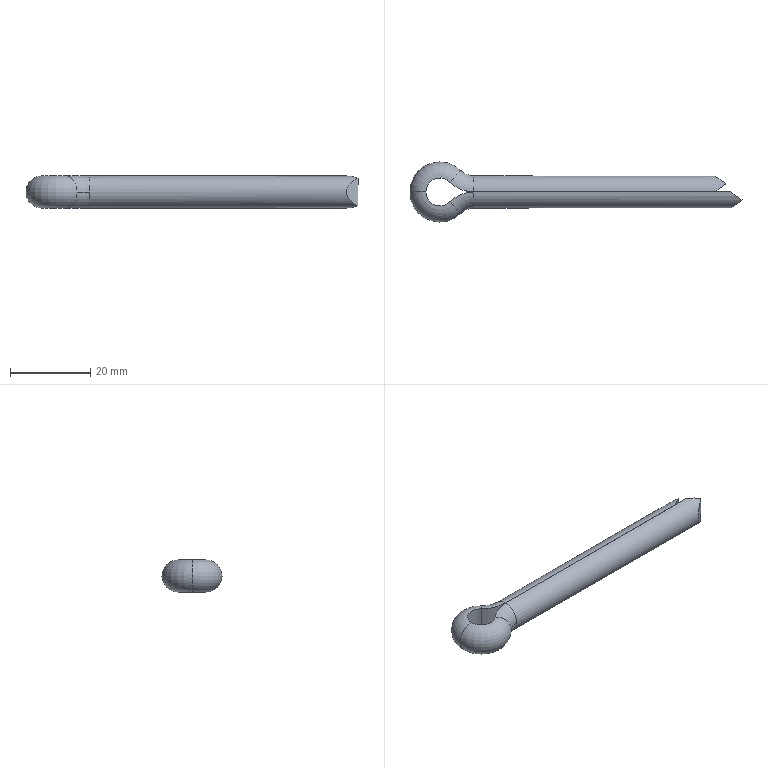Part | SolidWorks | features Cut 1, Sweep 1 | 1 solid | 17 faces | box 83 x 15 x 8 mm | volume 4081 mm3 | torus 6 | plane 6 | cylinder 5 | commonest cylinder face diameters 8 x2 17.139 x2 7.004 x1
STEP:
#1=CARTESIAN_POINT('',(0.,4.,0.));
#2=VERTEX_POINT('',#1);
#3=CARTESIAN_POINT('',(0.,0.002,4.));
#4=VERTEX_POINT('',#3);
#5=CARTESIAN_POINT('',(0.,0.,0.));
#6=DIRECTION('',(1.,0.,0.));
#7=DIRECTION('',(0.,0.,-1.));
#8=AXIS2_PLACEMENT_3D('',#5,#6,#7);
#9=CIRCLE('',#8,4.);
#10=EDGE_CURVE('',#2,#4,#9,.T.);
#11=ORIENTED_EDGE('',*,*,#10,.F.);
#12=CARTESIAN_POINT('',(-3.219,5.325,0.));
#13=VERTEX_POINT('',#12);
#14=CARTESIAN_POINT('',(0.,8.571,0.));
#15=DIRECTION('',(0.,0.,-1.));
#16=DIRECTION('',(-1.,0.,0.));
#17=AXIS2_PLACEMENT_3D('',#14,#15,#16);
#18=CIRCLE('',#17,4.571);
#19=EDGE_CURVE('',#2,#13,#18,.T.);
#20=ORIENTED_EDGE('',*,*,#19,.T.);
#21=CARTESIAN_POINT('',(-6.034,2.487,4.));
#22=VERTEX_POINT('',#21);
#23=CARTESIAN_POINT('',(-6.036,2.485,0.));
#24=DIRECTION('',(0.7101,-0.7041,0.));
#25=DIRECTION('',(0.,0.,-1.));
#26=AXIS2_PLACEMENT_3D('',#23,#24,#25);
#27=CIRCLE('',#26,4.);
#28=EDGE_CURVE('',#13,#22,#27,.T.);
#29=ORIENTED_EDGE('',*,*,#28,.T.);
#30=CARTESIAN_POINT('',(0.,8.571,4.));
#31=DIRECTION('',(0.,0.,-1.));
#32=DIRECTION('',(-1.,0.,0.));
#33=AXIS2_PLACEMENT_3D('',#30,#31,#32);
#34=CIRCLE('',#33,8.569);
#35=EDGE_CURVE('',#4,#22,#34,.T.);
#36=ORIENTED_EDGE('',*,*,#35,.F.);
#37=EDGE_LOOP('',(#11,#20,#29,#36));
#38=FACE_OUTER_BOUND('',#37,.T.);
#39=CARTESIAN_POINT('',(0.,8.571,0.));
#40=DIRECTION('',(0.,0.,-1.));
#41=DIRECTION('',(-1.,0.,0.));
#42=AXIS2_PLACEMENT_3D('',#39,#40,#41);
#43=TOROIDAL_SURFACE('',#42,8.571,4.);
#44=ADVANCED_FACE('',(#38),#43,.T.);
#45=CARTESIAN_POINT('',(-3.219,-5.325,0.));
#46=VERTEX_POINT('',#45);
#47=CARTESIAN_POINT('',(-6.034,-2.487,4.));
#48=VERTEX_POINT('',#47);
#49=CARTESIAN_POINT('',(-6.036,-2.485,0.));
#50=DIRECTION('',(-0.7101,-0.7041,0.));
#51=DIRECTION('',(0.,0.,-1.));
#52=AXIS2_PLACEMENT_3D('',#49,#50,#51);
#53=CIRCLE('',#52,4.);
#54=EDGE_CURVE('',#46,#48,#53,.T.);
#55=ORIENTED_EDGE('',*,*,#54,.F.);
#56=CARTESIAN_POINT('',(0.,-4.,0.));
#57=VERTEX_POINT('',#56);
#58=CARTESIAN_POINT('',(0.,-8.571,0.));
#59=DIRECTION('',(0.,0.,-1.));
#60=DIRECTION('',(-1.,0.,0.));
#61=AXIS2_PLACEMENT_3D('',#58,#59,#60);
#62=CIRCLE('',#61,4.571);
#63=EDGE_CURVE('',#46,#57,#62,.T.);
#64=ORIENTED_EDGE('',*,*,#63,.T.);
#65=CARTESIAN_POINT('',(0.,-0.002,4.));
#66=VERTEX_POINT('',#65);
#67=CARTESIAN_POINT('',(0.,0.,0.));
#68=DIRECTION('',(-1.,0.,0.));
#69=DIRECTION('',(0.,0.,-1.));
#70=AXIS2_PLACEMENT_3D('',#67,#68,#69);
#71=CIRCLE('',#70,4.);
#72=EDGE_CURVE('',#57,#66,#71,.T.);
#73=ORIENTED_EDGE('',*,*,#72,.T.);
#74=CARTESIAN_POINT('',(0.,-8.571,4.));
#75=DIRECTION('',(0.,0.,-1.));
#76=DIRECTION('',(-1.,0.,0.));
#77=AXIS2_PLACEMENT_3D('',#74,#75,#76);
#78=CIRCLE('',#77,8.569);
#79=EDGE_CURVE('',#48,#66,#78,.T.);
#80=ORIENTED_EDGE('',*,*,#79,.F.);
#81=EDGE_LOOP('',(#55,#64,#73,#80));
#82=FACE_OUTER_BOUND('',#81,.T.);
#83=CARTESIAN_POINT('',(0.,-8.571,0.));
#84=DIRECTION('',(0.,0.,-1.));
#85=DIRECTION('',(-1.,0.,0.));
#86=AXIS2_PLACEMENT_3D('',#83,#84,#85);
#87=TOROIDAL_SURFACE('',#86,8.571,4.);
#88=ADVANCED_FACE('',(#82),#87,.T.);
#89=CARTESIAN_POINT('',(-6.034,2.487,-4.));
#90=VERTEX_POINT('',#89);
#91=CARTESIAN_POINT('',(-12.002,0.,-4.));
#92=VERTEX_POINT('',#91);
#93=CARTESIAN_POINT('',(-8.5,0.,-4.));
#94=DIRECTION('',(0.,0.,1.));
#95=DIRECTION('',(1.,0.,0.));
#96=AXIS2_PLACEMENT_3D('',#93,#94,#95);
#97=CIRCLE('',#96,3.502);
#98=EDGE_CURVE('',#90,#92,#97,.T.);
#99=ORIENTED_EDGE('',*,*,#98,.T.);
#100=CARTESIAN_POINT('',(-12.002,0.,4.));
#101=VERTEX_POINT('',#100);
#102=CARTESIAN_POINT('',(-12.,0.,0.));
#103=DIRECTION('',(0.,1.,0.));
#104=DIRECTION('',(-1.,0.,0.));
#105=AXIS2_PLACEMENT_3D('',#102,#103,#104);
#106=CIRCLE('',#105,4.);
#107=EDGE_CURVE('',#92,#101,#106,.T.);
#108=ORIENTED_EDGE('',*,*,#107,.T.);
#109=CARTESIAN_POINT('',(-8.5,0.,4.));
#110=DIRECTION('',(0.,0.,1.));
#111=DIRECTION('',(1.,0.,0.));
#112=AXIS2_PLACEMENT_3D('',#109,#110,#111);
#113=CIRCLE('',#112,3.502);
#114=EDGE_CURVE('',#22,#101,#113,.T.);
#115=ORIENTED_EDGE('',*,*,#114,.F.);
#116=ORIENTED_EDGE('',*,*,#28,.F.);
#117=CARTESIAN_POINT('',(-6.036,2.485,0.));
#118=DIRECTION('',(0.7101,-0.7041,0.));
#119=DIRECTION('',(0.,0.,-1.));
#120=AXIS2_PLACEMENT_3D('',#117,#118,#119);
#121=CIRCLE('',#120,4.);
#122=EDGE_CURVE('',#90,#13,#121,.T.);
#123=ORIENTED_EDGE('',*,*,#122,.F.);
#124=EDGE_LOOP('',(#99,#108,#115,#116,#123));
#125=FACE_OUTER_BOUND('',#124,.T.);
#126=CARTESIAN_POINT('',(-8.5,0.,0.));
#127=DIRECTION('',(0.,0.,1.));
#128=DIRECTION('',(1.,0.,0.));
#129=AXIS2_PLACEMENT_3D('',#126,#127,#128);
#130=TOROIDAL_SURFACE('',#129,3.5,4.);
#131=ADVANCED_FACE('',(#125),#130,.T.);
#132=CARTESIAN_POINT('',(64.137,-0.002,4.));
#133=VERTEX_POINT('',#132);
#134=CARTESIAN_POINT('',(0.,-0.002,4.));
#135=DIRECTION('',(1.,0.,0.));
#136=VECTOR('',#135,1000.);
#137=LINE('',#134,#136);
#138=EDGE_CURVE('',#66,#133,#137,.T.);
#139=ORIENTED_EDGE('',*,*,#138,.T.);
#140=CARTESIAN_POINT('',(64.137,-0.002,-4.));
#141=VERTEX_POINT('',#140);
#142=CARTESIAN_POINT('',(64.137,-0.002,4.));
#143=DIRECTION('',(0.,0.,-1.));
#144=VECTOR('',#143,1000.);
#145=LINE('',#142,#144);
#146=EDGE_CURVE('',#133,#141,#145,.T.);
#147=ORIENTED_EDGE('',*,*,#146,.T.);
#148=CARTESIAN_POINT('',(0.,-0.002,-4.));
#149=VERTEX_POINT('',#148);
#150=CARTESIAN_POINT('',(0.,-0.002,-4.));
#151=DIRECTION('',(1.,0.,0.));
#152=VECTOR('',#151,1000.);
#153=LINE('',#150,#152);
#154=EDGE_CURVE('',#149,#141,#153,.T.);
#155=ORIENTED_EDGE('',*,*,#154,.F.);
#156=CARTESIAN_POINT('',(0.,-0.002,4.));
#157=DIRECTION('',(0.,0.,-1.));
#158=VECTOR('',#157,1000.);
#159=LINE('',#156,#158);
#160=EDGE_CURVE('',#66,#149,#159,.T.);
#161=ORIENTED_EDGE('',*,*,#160,.F.);
#162=EDGE_LOOP('',(#139,#147,#155,#161));
#163=FACE_OUTER_BOUND('',#162,.T.);
#164=CARTESIAN_POINT('',(0.,-0.002,4.));
#165=DIRECTION('',(0.,-1.,0.));
#166=DIRECTION('',(0.,0.,-1.));
#167=AXIS2_PLACEMENT_3D('',#164,#165,#166);
#168=PLANE('',#167);
#169=ADVANCED_FACE('',(#163),#168,.F.);
#170=CARTESIAN_POINT('',(67.,-2.001,-3.464));
#171=VERTEX_POINT('',#170);
#172=CARTESIAN_POINT('',(67.,-2.001,3.464));
#173=VERTEX_POINT('',#172);
#174=CARTESIAN_POINT('',(67.,-2.001,-3.464));
#175=CARTESIAN_POINT('',(62.731,-4.999,-1.731));
#176=CARTESIAN_POINT('',(62.731,-4.999,1.731));
#177=CARTESIAN_POINT('',(67.,-2.001,3.464));
#178=(BOUNDED_CURVE()B_SPLINE_CURVE(3,(#174,#175,#176,#177),.UNSPECIFIED.,.F.,.F.)B_SPLINE_CURVE_WITH_KNOTS((4,4),(2.095,4.189),.UNSPECIFIED.)CURVE()GEOMETRIC_REPRESENTATION_ITEM()RATIONAL_B_SPLINE_CURVE((1.,0.6668,0.6668,1.))REPRESENTATION_ITEM(''));
#179=EDGE_CURVE('',#171,#173,#178,.T.);
#180=ORIENTED_EDGE('',*,*,#179,.T.);
#181=CARTESIAN_POINT('',(67.,-2.001,3.464));
#182=CARTESIAN_POINT('',(66.124,-1.39,3.817));
#183=CARTESIAN_POINT('',(65.148,-0.7079,4.));
#184=CARTESIAN_POINT('',(64.137,-0.002,4.));
#185=(BOUNDED_CURVE()B_SPLINE_CURVE(3,(#181,#182,#183,#184),.UNSPECIFIED.,.F.,.F.)B_SPLINE_CURVE_WITH_KNOTS((4,4),(1.047,1.57),.UNSPECIFIED.)CURVE()GEOMETRIC_REPRESENTATION_ITEM()RATIONAL_B_SPLINE_CURVE((1.,0.9773,0.9773,1.))REPRESENTATION_ITEM(''));
#186=EDGE_CURVE('',#173,#133,#185,.T.);
#187=ORIENTED_EDGE('',*,*,#186,.T.);
#188=ORIENTED_EDGE('',*,*,#138,.F.);
#189=ORIENTED_EDGE('',*,*,#72,.F.);
#190=CARTESIAN_POINT('',(0.,0.,0.));
#191=DIRECTION('',(-1.,0.,0.));
#192=DIRECTION('',(0.,0.,-1.));
#193=AXIS2_PLACEMENT_3D('',#190,#191,#192);
#194=CIRCLE('',#193,4.);
#195=EDGE_CURVE('',#149,#57,#194,.T.);
#196=ORIENTED_EDGE('',*,*,#195,.F.);
#197=ORIENTED_EDGE('',*,*,#154,.T.);
#198=CARTESIAN_POINT('',(64.137,-0.002,-4.));
#199=CARTESIAN_POINT('',(65.148,-0.7079,-4.));
#200=CARTESIAN_POINT('',(66.124,-1.39,-3.817));
#201=CARTESIAN_POINT('',(67.,-2.001,-3.464));
#202=(BOUNDED_CURVE()B_SPLINE_CURVE(3,(#198,#199,#200,#201),.UNSPECIFIED.,.F.,.F.)B_SPLINE_CURVE_WITH_KNOTS((4,4),(4.713,5.236),.UNSPECIFIED.)CURVE()GEOMETRIC_REPRESENTATION_ITEM()RATIONAL_B_SPLINE_CURVE((1.,0.9773,0.9773,1.))REPRESENTATION_ITEM(''));
#203=EDGE_CURVE('',#141,#171,#202,.T.);
#204=ORIENTED_EDGE('',*,*,#203,.T.);
#205=EDGE_LOOP('',(#180,#187,#188,#189,#196,#197,#204));
#206=FACE_OUTER_BOUND('',#205,.T.);
#207=CARTESIAN_POINT('',(0.,0.,0.));
#208=DIRECTION('',(1.,0.,0.));
#209=DIRECTION('',(0.,0.,-1.));
#210=AXIS2_PLACEMENT_3D('',#207,#208,#209);
#211=CYLINDRICAL_SURFACE('',#210,4.);
#212=ADVANCED_FACE('',(#206),#211,.T.);
#213=CARTESIAN_POINT('',(-6.034,-2.487,-4.));
#214=VERTEX_POINT('',#213);
#215=CARTESIAN_POINT('',(-6.034,-2.487,4.));
#216=DIRECTION('',(0.,0.,-1.));
#217=VECTOR('',#216,1000.);
#218=LINE('',#215,#217);
#219=EDGE_CURVE('',#48,#214,#218,.T.);
#220=ORIENTED_EDGE('',*,*,#219,.F.);
#221=ORIENTED_EDGE('',*,*,#79,.T.);
#222=ORIENTED_EDGE('',*,*,#160,.T.);
#223=CARTESIAN_POINT('',(0.,-8.571,-4.));
#224=DIRECTION('',(0.,0.,-1.));
#225=DIRECTION('',(-1.,0.,0.));
#226=AXIS2_PLACEMENT_3D('',#223,#224,#225);
#227=CIRCLE('',#226,8.569);
#228=EDGE_CURVE('',#214,#149,#227,.T.);
#229=ORIENTED_EDGE('',*,*,#228,.F.);
#230=EDGE_LOOP('',(#220,#221,#222,#229));
#231=FACE_OUTER_BOUND('',#230,.T.);
#232=CARTESIAN_POINT('',(0.,-8.571,0.));
#233=DIRECTION('',(0.,0.,-1.));
#234=DIRECTION('',(-1.,0.,0.));
#235=AXIS2_PLACEMENT_3D('',#232,#233,#234);
#236=CYLINDRICAL_SURFACE('',#235,8.569);
#237=ADVANCED_FACE('',(#231),#236,.T.);
#238=ORIENTED_EDGE('',*,*,#63,.F.);
#239=CARTESIAN_POINT('',(-6.036,-2.485,0.));
#240=DIRECTION('',(-0.7101,-0.7041,0.));
#241=DIRECTION('',(0.,0.,-1.));
#242=AXIS2_PLACEMENT_3D('',#239,#240,#241);
#243=CIRCLE('',#242,4.);
#244=EDGE_CURVE('',#214,#46,#243,.T.);
#245=ORIENTED_EDGE('',*,*,#244,.F.);
#246=ORIENTED_EDGE('',*,*,#228,.T.);
#247=ORIENTED_EDGE('',*,*,#195,.T.);
#248=EDGE_LOOP('',(#238,#245,#246,#247));
#249=FACE_OUTER_BOUND('',#248,.T.);
#250=CARTESIAN_POINT('',(0.,-8.571,0.));
#251=DIRECTION('',(0.,0.,-1.));
#252=DIRECTION('',(-1.,0.,0.));
#253=AXIS2_PLACEMENT_3D('',#250,#251,#252);
#254=TOROIDAL_SURFACE('',#253,8.571,4.);
#255=ADVANCED_FACE('',(#249),#254,.T.);
#256=CARTESIAN_POINT('',(-6.034,2.487,4.));
#257=DIRECTION('',(0.,0.,-1.));
#258=VECTOR('',#257,1000.);
#259=LINE('',#256,#258);
#260=EDGE_CURVE('',#22,#90,#259,.T.);
#261=ORIENTED_EDGE('',*,*,#260,.F.);
#262=ORIENTED_EDGE('',*,*,#114,.T.);
#263=CARTESIAN_POINT('',(-8.5,0.,4.));
#264=DIRECTION('',(0.,0.,1.));
#265=DIRECTION('',(1.,0.,0.));
#266=AXIS2_PLACEMENT_3D('',#263,#264,#265);
#267=CIRCLE('',#266,3.502);
#268=EDGE_CURVE('',#101,#48,#267,.T.);
#269=ORIENTED_EDGE('',*,*,#268,.T.);
#270=ORIENTED_EDGE('',*,*,#219,.T.);
#271=CARTESIAN_POINT('',(-8.5,0.,-4.));
#272=DIRECTION('',(0.,0.,1.));
#273=DIRECTION('',(1.,0.,0.));
#274=AXIS2_PLACEMENT_3D('',#271,#272,#273);
#275=CIRCLE('',#274,3.502);
#276=EDGE_CURVE('',#92,#214,#275,.T.);
#277=ORIENTED_EDGE('',*,*,#276,.F.);
#278=ORIENTED_EDGE('',*,*,#98,.F.);
#279=EDGE_LOOP('',(#261,#262,#269,#270,#277,#278));
#280=FACE_OUTER_BOUND('',#279,.T.);
#281=CARTESIAN_POINT('',(-8.5,0.,0.));
#282=DIRECTION('',(0.,0.,1.));
#283=DIRECTION('',(1.,0.,0.));
#284=AXIS2_PLACEMENT_3D('',#281,#282,#283);
#285=CYLINDRICAL_SURFACE('',#284,3.502);
#286=ADVANCED_FACE('',(#280),#285,.F.);
#287=ORIENTED_EDGE('',*,*,#107,.F.);
#288=ORIENTED_EDGE('',*,*,#276,.T.);
#289=ORIENTED_EDGE('',*,*,#244,.T.);
#290=ORIENTED_EDGE('',*,*,#54,.T.);
#291=ORIENTED_EDGE('',*,*,#268,.F.);
#292=EDGE_LOOP('',(#287,#288,#289,#290,#291));
#293=FACE_OUTER_BOUND('',#292,.T.);
#294=CARTESIAN_POINT('',(-8.5,0.,0.));
#295=DIRECTION('',(0.,0.,1.));
#296=DIRECTION('',(1.,0.,0.));
#297=AXIS2_PLACEMENT_3D('',#294,#295,#296);
#298=TOROIDAL_SURFACE('',#297,3.5,4.);
#299=ADVANCED_FACE('',(#293),#298,.T.);
#300=CARTESIAN_POINT('',(0.,0.002,-4.));
#301=VERTEX_POINT('',#300);
#302=CARTESIAN_POINT('',(0.,0.002,4.));
#303=DIRECTION('',(0.,0.,-1.));
#304=VECTOR('',#303,1000.);
#305=LINE('',#302,#304);
#306=EDGE_CURVE('',#4,#301,#305,.T.);
#307=ORIENTED_EDGE('',*,*,#306,.F.);
#308=ORIENTED_EDGE('',*,*,#35,.T.);
#309=ORIENTED_EDGE('',*,*,#260,.T.);
#310=CARTESIAN_POINT('',(0.,8.571,-4.));
#311=DIRECTION('',(0.,0.,-1.));
#312=DIRECTION('',(-1.,0.,0.));
#313=AXIS2_PLACEMENT_3D('',#310,#311,#312);
#314=CIRCLE('',#313,8.569);
#315=EDGE_CURVE('',#301,#90,#314,.T.);
#316=ORIENTED_EDGE('',*,*,#315,.F.);
#317=EDGE_LOOP('',(#307,#308,#309,#316));
#318=FACE_OUTER_BOUND('',#317,.T.);
#319=CARTESIAN_POINT('',(0.,8.571,0.));
#320=DIRECTION('',(0.,0.,-1.));
#321=DIRECTION('',(-1.,0.,0.));
#322=AXIS2_PLACEMENT_3D('',#319,#320,#321);
#323=CYLINDRICAL_SURFACE('',#322,8.569);
#324=ADVANCED_FACE('',(#318),#323,.T.);
#325=ORIENTED_EDGE('',*,*,#19,.F.);
#326=CARTESIAN_POINT('',(0.,0.,0.));
#327=DIRECTION('',(1.,0.,0.));
#328=DIRECTION('',(0.,0.,-1.));
#329=AXIS2_PLACEMENT_3D('',#326,#327,#328);
#330=CIRCLE('',#329,4.);
#331=EDGE_CURVE('',#301,#2,#330,.T.);
#332=ORIENTED_EDGE('',*,*,#331,.F.);
#333=ORIENTED_EDGE('',*,*,#315,.T.);
#334=ORIENTED_EDGE('',*,*,#122,.T.);
#335=EDGE_LOOP('',(#325,#332,#333,#334));
#336=FACE_OUTER_BOUND('',#335,.T.);
#337=CARTESIAN_POINT('',(0.,8.571,0.));
#338=DIRECTION('',(0.,0.,-1.));
#339=DIRECTION('',(-1.,0.,0.));
#340=AXIS2_PLACEMENT_3D('',#337,#338,#339);
#341=TOROIDAL_SURFACE('',#340,8.571,4.);
#342=ADVANCED_FACE('',(#336),#341,.T.);
#343=CARTESIAN_POINT('',(63.,2.001,3.464));
#344=VERTEX_POINT('',#343);
#345=CARTESIAN_POINT('',(60.137,0.002,4.));
#346=VERTEX_POINT('',#345);
#347=CARTESIAN_POINT('',(63.,2.001,3.464));
#348=CARTESIAN_POINT('',(62.124,1.39,3.817));
#349=CARTESIAN_POINT('',(61.148,0.7079,4.));
#350=CARTESIAN_POINT('',(60.137,0.002,4.));
#351=(BOUNDED_CURVE()B_SPLINE_CURVE(3,(#347,#348,#349,#350),.UNSPECIFIED.,.F.,.F.)B_SPLINE_CURVE_WITH_KNOTS((4,4),(1.047,1.57),.UNSPECIFIED.)CURVE()GEOMETRIC_REPRESENTATION_ITEM()RATIONAL_B_SPLINE_CURVE((1.,0.9773,0.9773,1.))REPRESENTATION_ITEM(''));
#352=EDGE_CURVE('',#344,#346,#351,.T.);
#353=ORIENTED_EDGE('',*,*,#352,.F.);
#354=CARTESIAN_POINT('',(63.,2.001,-3.464));
#355=VERTEX_POINT('',#354);
#356=CARTESIAN_POINT('',(63.,2.001,-3.464));
#357=CARTESIAN_POINT('',(58.731,4.999,-1.731));
#358=CARTESIAN_POINT('',(58.731,4.999,1.731));
#359=CARTESIAN_POINT('',(63.,2.001,3.464));
#360=(BOUNDED_CURVE()B_SPLINE_CURVE(3,(#356,#357,#358,#359),.UNSPECIFIED.,.F.,.F.)B_SPLINE_CURVE_WITH_KNOTS((4,4),(2.095,4.189),.UNSPECIFIED.)CURVE()GEOMETRIC_REPRESENTATION_ITEM()RATIONAL_B_SPLINE_CURVE((1.,0.6668,0.6668,1.))REPRESENTATION_ITEM(''));
#361=EDGE_CURVE('',#355,#344,#360,.T.);
#362=ORIENTED_EDGE('',*,*,#361,.F.);
#363=CARTESIAN_POINT('',(60.137,0.002,-4.));
#364=VERTEX_POINT('',#363);
#365=CARTESIAN_POINT('',(60.137,0.002,-4.));
#366=CARTESIAN_POINT('',(61.148,0.7079,-4.));
#367=CARTESIAN_POINT('',(62.124,1.39,-3.817));
#368=CARTESIAN_POINT('',(63.,2.001,-3.464));
#369=(BOUNDED_CURVE()B_SPLINE_CURVE(3,(#365,#366,#367,#368),.UNSPECIFIED.,.F.,.F.)B_SPLINE_CURVE_WITH_KNOTS((4,4),(4.713,5.236),.UNSPECIFIED.)CURVE()GEOMETRIC_REPRESENTATION_ITEM()RATIONAL_B_SPLINE_CURVE((1.,0.9773,0.9773,1.))REPRESENTATION_ITEM(''));
#370=EDGE_CURVE('',#364,#355,#369,.T.);
#371=ORIENTED_EDGE('',*,*,#370,.F.);
#372=CARTESIAN_POINT('',(0.,0.002,-4.));
#373=DIRECTION('',(1.,0.,0.));
#374=VECTOR('',#373,1000.);
#375=LINE('',#372,#374);
#376=EDGE_CURVE('',#301,#364,#375,.T.);
#377=ORIENTED_EDGE('',*,*,#376,.F.);
#378=ORIENTED_EDGE('',*,*,#331,.T.);
#379=ORIENTED_EDGE('',*,*,#10,.T.);
#380=CARTESIAN_POINT('',(0.,0.002,4.));
#381=DIRECTION('',(1.,0.,0.));
#382=VECTOR('',#381,1000.);
#383=LINE('',#380,#382);
#384=EDGE_CURVE('',#4,#346,#383,.T.);
#385=ORIENTED_EDGE('',*,*,#384,.T.);
#386=EDGE_LOOP('',(#353,#362,#371,#377,#378,#379,#385));
#387=FACE_OUTER_BOUND('',#386,.T.);
#388=CARTESIAN_POINT('',(0.,0.,0.));
#389=DIRECTION('',(1.,0.,0.));
#390=DIRECTION('',(0.,0.,-1.));
#391=AXIS2_PLACEMENT_3D('',#388,#389,#390);
#392=CYLINDRICAL_SURFACE('',#391,4.);
#393=ADVANCED_FACE('',(#387),#392,.T.);
#394=CARTESIAN_POINT('',(60.137,0.002,4.));
#395=DIRECTION('',(0.,0.,-1.));
#396=VECTOR('',#395,1000.);
#397=LINE('',#394,#396);
#398=EDGE_CURVE('',#346,#364,#397,.T.);
#399=ORIENTED_EDGE('',*,*,#398,.F.);
#400=ORIENTED_EDGE('',*,*,#384,.F.);
#401=ORIENTED_EDGE('',*,*,#306,.T.);
#402=ORIENTED_EDGE('',*,*,#376,.T.);
#403=EDGE_LOOP('',(#399,#400,#401,#402));
#404=FACE_OUTER_BOUND('',#403,.T.);
#405=CARTESIAN_POINT('',(0.,0.002,4.));
#406=DIRECTION('',(0.,-1.,0.));
#407=DIRECTION('',(0.,0.,-1.));
#408=AXIS2_PLACEMENT_3D('',#405,#406,#407);
#409=PLANE('',#408);
#410=ADVANCED_FACE('',(#404),#409,.T.);
#411=ORIENTED_EDGE('',*,*,#352,.T.);
#412=ORIENTED_EDGE('',*,*,#398,.T.);
#413=ORIENTED_EDGE('',*,*,#370,.T.);
#414=CARTESIAN_POINT('',(63.,2.001,-4.));
#415=DIRECTION('',(0.,0.,1.));
#416=VECTOR('',#415,1000.);
#417=LINE('',#414,#416);
#418=EDGE_CURVE('',#355,#344,#417,.T.);
#419=ORIENTED_EDGE('',*,*,#418,.T.);
#420=EDGE_LOOP('',(#411,#412,#413,#419));
#421=FACE_OUTER_BOUND('',#420,.T.);
#422=CARTESIAN_POINT('',(63.,2.001,-4.));
#423=DIRECTION('',(-0.5724,0.82,0.));
#424=DIRECTION('',(-0.82,-0.5724,0.));
#425=AXIS2_PLACEMENT_3D('',#422,#423,#424);
#426=PLANE('',#425);
#427=ADVANCED_FACE('',(#421),#426,.F.);
#428=ORIENTED_EDGE('',*,*,#361,.T.);
#429=ORIENTED_EDGE('',*,*,#418,.F.);
#430=EDGE_LOOP('',(#428,#429));
#431=FACE_OUTER_BOUND('',#430,.T.);
#432=CARTESIAN_POINT('',(63.,2.001,-4.));
#433=DIRECTION('',(-0.5747,-0.8184,0.));
#434=DIRECTION('',(0.8184,-0.5747,0.));
#435=AXIS2_PLACEMENT_3D('',#432,#433,#434);
#436=PLANE('',#435);
#437=ADVANCED_FACE('',(#431),#436,.F.);
#438=CARTESIAN_POINT('',(67.,-2.001,-4.));
#439=DIRECTION('',(0.,0.,1.));
#440=VECTOR('',#439,1000.);
#441=LINE('',#438,#440);
#442=EDGE_CURVE('',#171,#173,#441,.T.);
#443=ORIENTED_EDGE('',*,*,#442,.T.);
#444=ORIENTED_EDGE('',*,*,#179,.F.);
#445=EDGE_LOOP('',(#443,#444));
#446=FACE_OUTER_BOUND('',#445,.T.);
#447=CARTESIAN_POINT('',(67.,-2.001,-4.));
#448=DIRECTION('',(-0.5747,0.8184,0.));
#449=DIRECTION('',(-0.8184,-0.5747,0.));
#450=AXIS2_PLACEMENT_3D('',#447,#448,#449);
#451=PLANE('',#450);
#452=ADVANCED_FACE('',(#446),#451,.F.);
#453=ORIENTED_EDGE('',*,*,#442,.F.);
#454=ORIENTED_EDGE('',*,*,#203,.F.);
#455=ORIENTED_EDGE('',*,*,#146,.F.);
#456=ORIENTED_EDGE('',*,*,#186,.F.);
#457=EDGE_LOOP('',(#453,#454,#455,#456));
#458=FACE_OUTER_BOUND('',#457,.T.);
#459=CARTESIAN_POINT('',(67.,-2.001,-4.));
#460=DIRECTION('',(-0.5724,-0.82,0.));
#461=DIRECTION('',(0.82,-0.5724,0.));
#462=AXIS2_PLACEMENT_3D('',#459,#460,#461);
#463=PLANE('',#462);
#464=ADVANCED_FACE('',(#458),#463,.F.);
#465=CLOSED_SHELL('',(#44,#88,#131,#169,#212,#237,#255,#286,#299,#324,#342,#393,#410,#427,#437,#452,#464));
#466=MANIFOLD_SOLID_BREP('',#465);
#467=CARTESIAN_POINT('',(0.,0.,0.));
#468=DIRECTION('',(0.,0.,1.));
#469=DIRECTION('',(1.,0.,0.));
#470=AXIS2_PLACEMENT_3D('',#467,#468,#469);
#471=(LENGTH_UNIT()NAMED_UNIT(*)SI_UNIT(.MILLI.,.METRE.));
#472=UNCERTAINTY_MEASURE_WITH_UNIT(LENGTH_MEASURE(0.00001),#471,'','');
#473=(NAMED_UNIT(*)PLANE_ANGLE_UNIT()SI_UNIT($,.RADIAN.));
#474=(NAMED_UNIT(*)SI_UNIT($,.STERADIAN.)SOLID_ANGLE_UNIT());
#475=(GEOMETRIC_REPRESENTATION_CONTEXT(3)GLOBAL_UNCERTAINTY_ASSIGNED_CONTEXT((#472))GLOBAL_UNIT_ASSIGNED_CONTEXT((#471,#473,#474))REPRESENTATION_CONTEXT('',''));
#476=ADVANCED_BREP_SHAPE_REPRESENTATION('',(#466,#470),#475);